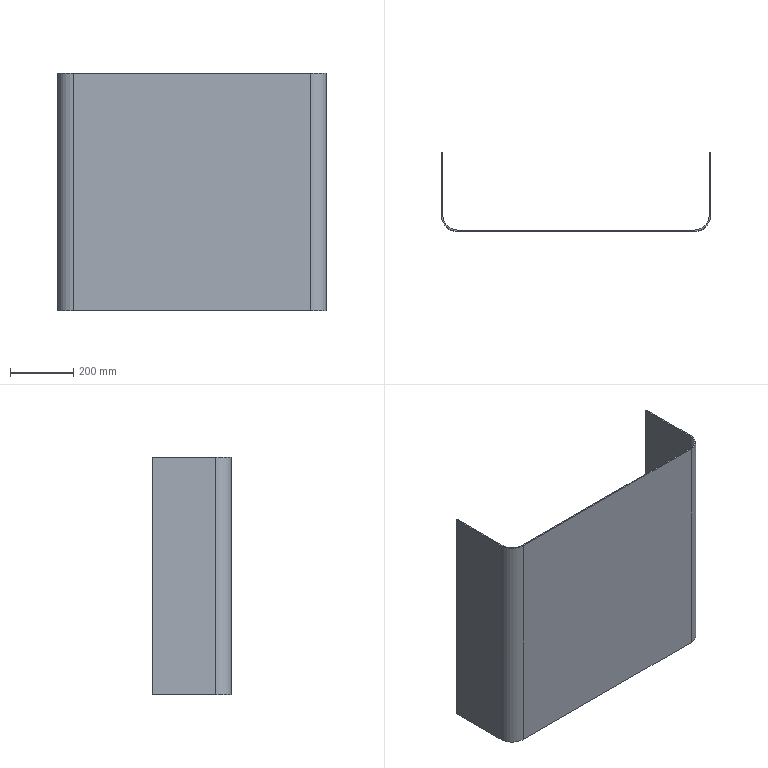Part | SolidWorks | features BaseBody 1 | 1 solid | 14 faces | box 850 x 250 x 750 mm | volume 3902389 mm3 | plane 10 | cylinder 4 | commonest cylinder face diameters 92 x2 100 x2
STEP:
#1=CARTESIAN_POINT('',(375.,0.,0.));
#2=VERTEX_POINT('',#1);
#3=CARTESIAN_POINT('',(375.,0.,750.));
#4=VERTEX_POINT('',#3);
#5=CARTESIAN_POINT('',(375.,0.,375.));
#6=DIRECTION('',(0.,0.,1.));
#7=VECTOR('',#6,1000.);
#8=LINE('',#5,#7);
#9=EDGE_CURVE('',#2,#4,#8,.T.);
#10=ORIENTED_EDGE('',*,*,#9,.T.);
#11=CARTESIAN_POINT('',(-375.,0.,750.));
#12=VERTEX_POINT('',#11);
#13=CARTESIAN_POINT('',(0.,0.,750.));
#14=DIRECTION('',(-1.,0.,0.));
#15=VECTOR('',#14,1000.);
#16=LINE('',#13,#15);
#17=EDGE_CURVE('',#4,#12,#16,.T.);
#18=ORIENTED_EDGE('',*,*,#17,.T.);
#19=CARTESIAN_POINT('',(-375.,0.,0.));
#20=VERTEX_POINT('',#19);
#21=CARTESIAN_POINT('',(-375.,0.,375.));
#22=DIRECTION('',(0.,0.,-1.));
#23=VECTOR('',#22,1000.);
#24=LINE('',#21,#23);
#25=EDGE_CURVE('',#12,#20,#24,.T.);
#26=ORIENTED_EDGE('',*,*,#25,.T.);
#27=CARTESIAN_POINT('',(0.,0.,0.));
#28=DIRECTION('',(1.,0.,0.));
#29=VECTOR('',#28,1000.);
#30=LINE('',#27,#29);
#31=EDGE_CURVE('',#20,#2,#30,.T.);
#32=ORIENTED_EDGE('',*,*,#31,.T.);
#33=EDGE_LOOP('',(#10,#18,#26,#32));
#34=FACE_OUTER_BOUND('',#33,.T.);
#35=CARTESIAN_POINT('',(0.,0.,375.));
#36=DIRECTION('',(0.,-1.,0.));
#37=DIRECTION('',(1.,0.,0.));
#38=AXIS2_PLACEMENT_3D('',#35,#36,#37);
#39=PLANE('',#38);
#40=ADVANCED_FACE('',(#34),#39,.T.);
#41=ORIENTED_EDGE('',*,*,#17,.F.);
#42=CARTESIAN_POINT('',(425.,50.,750.));
#43=VERTEX_POINT('',#42);
#44=CARTESIAN_POINT('',(375.,50.,750.));
#45=DIRECTION('',(0.,0.,-1.));
#46=DIRECTION('',(-1.,0.,0.));
#47=AXIS2_PLACEMENT_3D('',#44,#45,#46);
#48=CIRCLE('',#47,50.);
#49=EDGE_CURVE('',#43,#4,#48,.T.);
#50=ORIENTED_EDGE('',*,*,#49,.F.);
#51=CARTESIAN_POINT('',(425.,250.,750.));
#52=VERTEX_POINT('',#51);
#53=CARTESIAN_POINT('',(425.,-400.021,750.));
#54=DIRECTION('',(0.,-1.,0.));
#55=VECTOR('',#54,1000.);
#56=LINE('',#53,#55);
#57=EDGE_CURVE('',#52,#43,#56,.T.);
#58=ORIENTED_EDGE('',*,*,#57,.F.);
#59=CARTESIAN_POINT('',(421.,250.,750.));
#60=VERTEX_POINT('',#59);
#61=CARTESIAN_POINT('',(421.,250.,750.));
#62=DIRECTION('',(-1.,0.,0.));
#63=VECTOR('',#62,1000.);
#64=LINE('',#61,#63);
#65=EDGE_CURVE('',#52,#60,#64,.T.);
#66=ORIENTED_EDGE('',*,*,#65,.T.);
#67=CARTESIAN_POINT('',(421.,50.,750.));
#68=VERTEX_POINT('',#67);
#69=CARTESIAN_POINT('',(421.,50.,750.));
#70=DIRECTION('',(0.,-1.,0.));
#71=VECTOR('',#70,1000.);
#72=LINE('',#69,#71);
#73=EDGE_CURVE('',#60,#68,#72,.T.);
#74=ORIENTED_EDGE('',*,*,#73,.T.);
#75=CARTESIAN_POINT('',(375.,4.,750.));
#76=VERTEX_POINT('',#75);
#77=CARTESIAN_POINT('',(375.,50.,750.));
#78=DIRECTION('',(0.,0.,-1.));
#79=DIRECTION('',(-1.,0.,0.));
#80=AXIS2_PLACEMENT_3D('',#77,#78,#79);
#81=CIRCLE('',#80,46.);
#82=EDGE_CURVE('',#68,#76,#81,.T.);
#83=ORIENTED_EDGE('',*,*,#82,.T.);
#84=CARTESIAN_POINT('',(-375.,4.,750.));
#85=VERTEX_POINT('',#84);
#86=CARTESIAN_POINT('',(450.021,4.,750.));
#87=DIRECTION('',(-1.,0.,0.));
#88=VECTOR('',#87,1000.);
#89=LINE('',#86,#88);
#90=EDGE_CURVE('',#76,#85,#89,.T.);
#91=ORIENTED_EDGE('',*,*,#90,.T.);
#92=CARTESIAN_POINT('',(-421.,50.,750.));
#93=VERTEX_POINT('',#92);
#94=CARTESIAN_POINT('',(-375.,50.,750.));
#95=DIRECTION('',(0.,0.,-1.));
#96=DIRECTION('',(-1.,0.,0.));
#97=AXIS2_PLACEMENT_3D('',#94,#95,#96);
#98=CIRCLE('',#97,46.);
#99=EDGE_CURVE('',#85,#93,#98,.T.);
#100=ORIENTED_EDGE('',*,*,#99,.T.);
#101=CARTESIAN_POINT('',(-421.,250.,750.));
#102=VERTEX_POINT('',#101);
#103=CARTESIAN_POINT('',(-421.,-850.042,750.));
#104=DIRECTION('',(0.,1.,0.));
#105=VECTOR('',#104,1000.);
#106=LINE('',#103,#105);
#107=EDGE_CURVE('',#93,#102,#106,.T.);
#108=ORIENTED_EDGE('',*,*,#107,.T.);
#109=CARTESIAN_POINT('',(-425.,250.,750.));
#110=VERTEX_POINT('',#109);
#111=CARTESIAN_POINT('',(-421.,250.,750.));
#112=DIRECTION('',(-1.,0.,0.));
#113=VECTOR('',#112,1000.);
#114=LINE('',#111,#113);
#115=EDGE_CURVE('',#102,#110,#114,.T.);
#116=ORIENTED_EDGE('',*,*,#115,.T.);
#117=CARTESIAN_POINT('',(-425.,50.,750.));
#118=VERTEX_POINT('',#117);
#119=CARTESIAN_POINT('',(-425.,-400.021,750.));
#120=DIRECTION('',(0.,1.,0.));
#121=VECTOR('',#120,1000.);
#122=LINE('',#119,#121);
#123=EDGE_CURVE('',#118,#110,#122,.T.);
#124=ORIENTED_EDGE('',*,*,#123,.F.);
#125=CARTESIAN_POINT('',(-375.,50.,750.));
#126=DIRECTION('',(0.,0.,-1.));
#127=DIRECTION('',(-1.,0.,0.));
#128=AXIS2_PLACEMENT_3D('',#125,#126,#127);
#129=CIRCLE('',#128,50.);
#130=EDGE_CURVE('',#12,#118,#129,.T.);
#131=ORIENTED_EDGE('',*,*,#130,.F.);
#132=EDGE_LOOP('',(#41,#50,#58,#66,#74,#83,#91,#100,#108,#116,#124,#131));
#133=FACE_OUTER_BOUND('',#132,.T.);
#134=CARTESIAN_POINT('',(450.021,4.,750.));
#135=DIRECTION('',(0.,0.,1.));
#136=DIRECTION('',(1.,0.,0.));
#137=AXIS2_PLACEMENT_3D('',#134,#135,#136);
#138=PLANE('',#137);
#139=ADVANCED_FACE('',(#133),#138,.T.);
#140=CARTESIAN_POINT('',(425.,50.,0.));
#141=VERTEX_POINT('',#140);
#142=CARTESIAN_POINT('',(425.,50.,375.));
#143=DIRECTION('',(0.,0.,1.));
#144=VECTOR('',#143,1000.);
#145=LINE('',#142,#144);
#146=EDGE_CURVE('',#141,#43,#145,.T.);
#147=ORIENTED_EDGE('',*,*,#146,.T.);
#148=ORIENTED_EDGE('',*,*,#49,.T.);
#149=ORIENTED_EDGE('',*,*,#9,.F.);
#150=CARTESIAN_POINT('',(375.,50.,0.));
#151=DIRECTION('',(0.,0.,1.));
#152=DIRECTION('',(-1.,0.,0.));
#153=AXIS2_PLACEMENT_3D('',#150,#151,#152);
#154=CIRCLE('',#153,50.);
#155=EDGE_CURVE('',#2,#141,#154,.T.);
#156=ORIENTED_EDGE('',*,*,#155,.T.);
#157=EDGE_LOOP('',(#147,#148,#149,#156));
#158=FACE_OUTER_BOUND('',#157,.T.);
#159=CARTESIAN_POINT('',(375.,50.,375.));
#160=DIRECTION('',(0.,0.,-1.));
#161=DIRECTION('',(-1.,0.,0.));
#162=AXIS2_PLACEMENT_3D('',#159,#160,#161);
#163=CYLINDRICAL_SURFACE('',#162,50.);
#164=ADVANCED_FACE('',(#158),#163,.T.);
#165=CARTESIAN_POINT('',(-375.,4.,0.));
#166=VERTEX_POINT('',#165);
#167=CARTESIAN_POINT('',(375.,4.,0.));
#168=VERTEX_POINT('',#167);
#169=CARTESIAN_POINT('',(-450.021,4.,0.));
#170=DIRECTION('',(1.,0.,0.));
#171=VECTOR('',#170,1000.);
#172=LINE('',#169,#171);
#173=EDGE_CURVE('',#166,#168,#172,.T.);
#174=ORIENTED_EDGE('',*,*,#173,.T.);
#175=CARTESIAN_POINT('',(421.,50.,0.));
#176=VERTEX_POINT('',#175);
#177=CARTESIAN_POINT('',(375.,50.,0.));
#178=DIRECTION('',(0.,0.,1.));
#179=DIRECTION('',(-1.,0.,0.));
#180=AXIS2_PLACEMENT_3D('',#177,#178,#179);
#181=CIRCLE('',#180,46.);
#182=EDGE_CURVE('',#168,#176,#181,.T.);
#183=ORIENTED_EDGE('',*,*,#182,.T.);
#184=CARTESIAN_POINT('',(421.,250.,0.));
#185=VERTEX_POINT('',#184);
#186=CARTESIAN_POINT('',(421.,-850.042,0.));
#187=DIRECTION('',(0.,1.,0.));
#188=VECTOR('',#187,1000.);
#189=LINE('',#186,#188);
#190=EDGE_CURVE('',#176,#185,#189,.T.);
#191=ORIENTED_EDGE('',*,*,#190,.T.);
#192=CARTESIAN_POINT('',(425.,250.,0.));
#193=VERTEX_POINT('',#192);
#194=CARTESIAN_POINT('',(421.,250.,0.));
#195=DIRECTION('',(-1.,0.,0.));
#196=VECTOR('',#195,1000.);
#197=LINE('',#194,#196);
#198=EDGE_CURVE('',#193,#185,#197,.T.);
#199=ORIENTED_EDGE('',*,*,#198,.F.);
#200=CARTESIAN_POINT('',(425.,-400.021,0.));
#201=DIRECTION('',(0.,1.,0.));
#202=VECTOR('',#201,1000.);
#203=LINE('',#200,#202);
#204=EDGE_CURVE('',#141,#193,#203,.T.);
#205=ORIENTED_EDGE('',*,*,#204,.F.);
#206=ORIENTED_EDGE('',*,*,#155,.F.);
#207=ORIENTED_EDGE('',*,*,#31,.F.);
#208=CARTESIAN_POINT('',(-425.,50.,0.));
#209=VERTEX_POINT('',#208);
#210=CARTESIAN_POINT('',(-375.,50.,0.));
#211=DIRECTION('',(0.,0.,1.));
#212=DIRECTION('',(-1.,0.,0.));
#213=AXIS2_PLACEMENT_3D('',#210,#211,#212);
#214=CIRCLE('',#213,50.);
#215=EDGE_CURVE('',#209,#20,#214,.T.);
#216=ORIENTED_EDGE('',*,*,#215,.F.);
#217=CARTESIAN_POINT('',(-425.,250.,0.));
#218=VERTEX_POINT('',#217);
#219=CARTESIAN_POINT('',(-425.,-400.021,0.));
#220=DIRECTION('',(0.,-1.,0.));
#221=VECTOR('',#220,1000.);
#222=LINE('',#219,#221);
#223=EDGE_CURVE('',#218,#209,#222,.T.);
#224=ORIENTED_EDGE('',*,*,#223,.F.);
#225=CARTESIAN_POINT('',(-421.,250.,0.));
#226=VERTEX_POINT('',#225);
#227=CARTESIAN_POINT('',(-421.,250.,0.));
#228=DIRECTION('',(1.,0.,0.));
#229=VECTOR('',#228,1000.);
#230=LINE('',#227,#229);
#231=EDGE_CURVE('',#218,#226,#230,.T.);
#232=ORIENTED_EDGE('',*,*,#231,.T.);
#233=CARTESIAN_POINT('',(-421.,50.,0.));
#234=VERTEX_POINT('',#233);
#235=CARTESIAN_POINT('',(-421.,50.,0.));
#236=DIRECTION('',(0.,-1.,0.));
#237=VECTOR('',#236,1000.);
#238=LINE('',#235,#237);
#239=EDGE_CURVE('',#226,#234,#238,.T.);
#240=ORIENTED_EDGE('',*,*,#239,.T.);
#241=CARTESIAN_POINT('',(-375.,50.,0.));
#242=DIRECTION('',(0.,0.,1.));
#243=DIRECTION('',(-1.,0.,0.));
#244=AXIS2_PLACEMENT_3D('',#241,#242,#243);
#245=CIRCLE('',#244,46.);
#246=EDGE_CURVE('',#234,#166,#245,.T.);
#247=ORIENTED_EDGE('',*,*,#246,.T.);
#248=EDGE_LOOP('',(#174,#183,#191,#199,#205,#206,#207,#216,#224,#232,#240,#247));
#249=FACE_OUTER_BOUND('',#248,.T.);
#250=CARTESIAN_POINT('',(-450.021,4.,0.));
#251=DIRECTION('',(0.,0.,-1.));
#252=DIRECTION('',(-1.,0.,0.));
#253=AXIS2_PLACEMENT_3D('',#250,#251,#252);
#254=PLANE('',#253);
#255=ADVANCED_FACE('',(#249),#254,.T.);
#256=ORIENTED_EDGE('',*,*,#25,.F.);
#257=ORIENTED_EDGE('',*,*,#130,.T.);
#258=CARTESIAN_POINT('',(-425.,50.,375.));
#259=DIRECTION('',(0.,0.,-1.));
#260=VECTOR('',#259,1000.);
#261=LINE('',#258,#260);
#262=EDGE_CURVE('',#118,#209,#261,.T.);
#263=ORIENTED_EDGE('',*,*,#262,.T.);
#264=ORIENTED_EDGE('',*,*,#215,.T.);
#265=EDGE_LOOP('',(#256,#257,#263,#264));
#266=FACE_OUTER_BOUND('',#265,.T.);
#267=CARTESIAN_POINT('',(-375.,50.,375.));
#268=DIRECTION('',(0.,0.,-1.));
#269=DIRECTION('',(-1.,0.,0.));
#270=AXIS2_PLACEMENT_3D('',#267,#268,#269);
#271=CYLINDRICAL_SURFACE('',#270,50.);
#272=ADVANCED_FACE('',(#266),#271,.T.);
#273=ORIENTED_EDGE('',*,*,#90,.F.);
#274=CARTESIAN_POINT('',(375.,4.,375.));
#275=DIRECTION('',(0.,0.,1.));
#276=VECTOR('',#275,1000.);
#277=LINE('',#274,#276);
#278=EDGE_CURVE('',#168,#76,#277,.T.);
#279=ORIENTED_EDGE('',*,*,#278,.F.);
#280=ORIENTED_EDGE('',*,*,#173,.F.);
#281=CARTESIAN_POINT('',(-375.,4.,375.));
#282=DIRECTION('',(0.,0.,-1.));
#283=VECTOR('',#282,1000.);
#284=LINE('',#281,#283);
#285=EDGE_CURVE('',#85,#166,#284,.T.);
#286=ORIENTED_EDGE('',*,*,#285,.F.);
#287=EDGE_LOOP('',(#273,#279,#280,#286));
#288=FACE_OUTER_BOUND('',#287,.T.);
#289=CARTESIAN_POINT('',(0.,4.,375.));
#290=DIRECTION('',(0.,-1.,0.));
#291=DIRECTION('',(1.,0.,0.));
#292=AXIS2_PLACEMENT_3D('',#289,#290,#291);
#293=PLANE('',#292);
#294=ADVANCED_FACE('',(#288),#293,.F.);
#295=CARTESIAN_POINT('',(425.,250.,375.));
#296=DIRECTION('',(0.,0.,1.));
#297=VECTOR('',#296,1000.);
#298=LINE('',#295,#297);
#299=EDGE_CURVE('',#193,#52,#298,.T.);
#300=ORIENTED_EDGE('',*,*,#299,.T.);
#301=ORIENTED_EDGE('',*,*,#57,.T.);
#302=ORIENTED_EDGE('',*,*,#146,.F.);
#303=ORIENTED_EDGE('',*,*,#204,.T.);
#304=EDGE_LOOP('',(#300,#301,#302,#303));
#305=FACE_OUTER_BOUND('',#304,.T.);
#306=CARTESIAN_POINT('',(425.,-400.021,375.));
#307=DIRECTION('',(1.,0.,0.));
#308=DIRECTION('',(0.,1.,0.));
#309=AXIS2_PLACEMENT_3D('',#306,#307,#308);
#310=PLANE('',#309);
#311=ADVANCED_FACE('',(#305),#310,.T.);
#312=CARTESIAN_POINT('',(-425.,250.,375.));
#313=DIRECTION('',(0.,0.,-1.));
#314=VECTOR('',#313,1000.);
#315=LINE('',#312,#314);
#316=EDGE_CURVE('',#110,#218,#315,.T.);
#317=ORIENTED_EDGE('',*,*,#316,.T.);
#318=ORIENTED_EDGE('',*,*,#223,.T.);
#319=ORIENTED_EDGE('',*,*,#262,.F.);
#320=ORIENTED_EDGE('',*,*,#123,.T.);
#321=EDGE_LOOP('',(#317,#318,#319,#320));
#322=FACE_OUTER_BOUND('',#321,.T.);
#323=CARTESIAN_POINT('',(-425.,-400.021,375.));
#324=DIRECTION('',(-1.,0.,0.));
#325=DIRECTION('',(0.,-1.,0.));
#326=AXIS2_PLACEMENT_3D('',#323,#324,#325);
#327=PLANE('',#326);
#328=ADVANCED_FACE('',(#322),#327,.T.);
#329=ORIENTED_EDGE('',*,*,#99,.F.);
#330=ORIENTED_EDGE('',*,*,#285,.T.);
#331=ORIENTED_EDGE('',*,*,#246,.F.);
#332=CARTESIAN_POINT('',(-421.,50.,375.));
#333=DIRECTION('',(0.,0.,-1.));
#334=VECTOR('',#333,1000.);
#335=LINE('',#332,#334);
#336=EDGE_CURVE('',#93,#234,#335,.T.);
#337=ORIENTED_EDGE('',*,*,#336,.F.);
#338=EDGE_LOOP('',(#329,#330,#331,#337));
#339=FACE_OUTER_BOUND('',#338,.T.);
#340=CARTESIAN_POINT('',(-375.,50.,375.));
#341=DIRECTION('',(0.,0.,-1.));
#342=DIRECTION('',(-1.,0.,0.));
#343=AXIS2_PLACEMENT_3D('',#340,#341,#342);
#344=CYLINDRICAL_SURFACE('',#343,46.);
#345=ADVANCED_FACE('',(#339),#344,.F.);
#346=ORIENTED_EDGE('',*,*,#82,.F.);
#347=CARTESIAN_POINT('',(421.,50.,375.));
#348=DIRECTION('',(0.,0.,1.));
#349=VECTOR('',#348,1000.);
#350=LINE('',#347,#349);
#351=EDGE_CURVE('',#176,#68,#350,.T.);
#352=ORIENTED_EDGE('',*,*,#351,.F.);
#353=ORIENTED_EDGE('',*,*,#182,.F.);
#354=ORIENTED_EDGE('',*,*,#278,.T.);
#355=EDGE_LOOP('',(#346,#352,#353,#354));
#356=FACE_OUTER_BOUND('',#355,.T.);
#357=CARTESIAN_POINT('',(375.,50.,375.));
#358=DIRECTION('',(0.,0.,-1.));
#359=DIRECTION('',(-1.,0.,0.));
#360=AXIS2_PLACEMENT_3D('',#357,#358,#359);
#361=CYLINDRICAL_SURFACE('',#360,46.);
#362=ADVANCED_FACE('',(#356),#361,.F.);
#363=CARTESIAN_POINT('',(421.,250.,750.));
#364=DIRECTION('',(0.,0.,1.));
#365=VECTOR('',#364,1000.);
#366=LINE('',#363,#365);
#367=EDGE_CURVE('',#185,#60,#366,.T.);
#368=ORIENTED_EDGE('',*,*,#367,.T.);
#369=ORIENTED_EDGE('',*,*,#65,.F.);
#370=ORIENTED_EDGE('',*,*,#299,.F.);
#371=ORIENTED_EDGE('',*,*,#198,.T.);
#372=EDGE_LOOP('',(#368,#369,#370,#371));
#373=FACE_OUTER_BOUND('',#372,.T.);
#374=CARTESIAN_POINT('',(421.,250.,750.));
#375=DIRECTION('',(0.,1.,0.));
#376=DIRECTION('',(0.,0.,1.));
#377=AXIS2_PLACEMENT_3D('',#374,#375,#376);
#378=PLANE('',#377);
#379=ADVANCED_FACE('',(#373),#378,.T.);
#380=CARTESIAN_POINT('',(-421.,250.,0.));
#381=DIRECTION('',(0.,0.,-1.));
#382=VECTOR('',#381,1000.);
#383=LINE('',#380,#382);
#384=EDGE_CURVE('',#102,#226,#383,.T.);
#385=ORIENTED_EDGE('',*,*,#384,.T.);
#386=ORIENTED_EDGE('',*,*,#231,.F.);
#387=ORIENTED_EDGE('',*,*,#316,.F.);
#388=ORIENTED_EDGE('',*,*,#115,.F.);
#389=EDGE_LOOP('',(#385,#386,#387,#388));
#390=FACE_OUTER_BOUND('',#389,.T.);
#391=CARTESIAN_POINT('',(-421.,250.,0.));
#392=DIRECTION('',(0.,1.,0.));
#393=DIRECTION('',(-1.,0.,0.));
#394=AXIS2_PLACEMENT_3D('',#391,#392,#393);
#395=PLANE('',#394);
#396=ADVANCED_FACE('',(#390),#395,.T.);
#397=ORIENTED_EDGE('',*,*,#239,.F.);
#398=ORIENTED_EDGE('',*,*,#384,.F.);
#399=ORIENTED_EDGE('',*,*,#107,.F.);
#400=ORIENTED_EDGE('',*,*,#336,.T.);
#401=EDGE_LOOP('',(#397,#398,#399,#400));
#402=FACE_OUTER_BOUND('',#401,.T.);
#403=CARTESIAN_POINT('',(-421.,-400.021,375.));
#404=DIRECTION('',(-1.,0.,0.));
#405=DIRECTION('',(0.,-1.,0.));
#406=AXIS2_PLACEMENT_3D('',#403,#404,#405);
#407=PLANE('',#406);
#408=ADVANCED_FACE('',(#402),#407,.F.);
#409=ORIENTED_EDGE('',*,*,#73,.F.);
#410=ORIENTED_EDGE('',*,*,#367,.F.);
#411=ORIENTED_EDGE('',*,*,#190,.F.);
#412=ORIENTED_EDGE('',*,*,#351,.T.);
#413=EDGE_LOOP('',(#409,#410,#411,#412));
#414=FACE_OUTER_BOUND('',#413,.T.);
#415=CARTESIAN_POINT('',(421.,-400.021,375.));
#416=DIRECTION('',(1.,0.,0.));
#417=DIRECTION('',(0.,1.,0.));
#418=AXIS2_PLACEMENT_3D('',#415,#416,#417);
#419=PLANE('',#418);
#420=ADVANCED_FACE('',(#414),#419,.F.);
#421=CLOSED_SHELL('',(#40,#139,#164,#255,#272,#294,#311,#328,#345,#362,#379,#396,#408,#420));
#422=MANIFOLD_SOLID_BREP('',#421);
#423=CARTESIAN_POINT('',(0.,0.,0.));
#424=DIRECTION('',(0.,0.,1.));
#425=DIRECTION('',(1.,0.,0.));
#426=AXIS2_PLACEMENT_3D('',#423,#424,#425);
#427=(LENGTH_UNIT()NAMED_UNIT(*)SI_UNIT(.MILLI.,.METRE.));
#428=UNCERTAINTY_MEASURE_WITH_UNIT(LENGTH_MEASURE(0.00001),#427,'','');
#429=(NAMED_UNIT(*)PLANE_ANGLE_UNIT()SI_UNIT($,.RADIAN.));
#430=(NAMED_UNIT(*)SI_UNIT($,.STERADIAN.)SOLID_ANGLE_UNIT());
#431=(GEOMETRIC_REPRESENTATION_CONTEXT(3)GLOBAL_UNCERTAINTY_ASSIGNED_CONTEXT((#428))GLOBAL_UNIT_ASSIGNED_CONTEXT((#427,#429,#430))REPRESENTATION_CONTEXT('',''));
#432=ADVANCED_BREP_SHAPE_REPRESENTATION('',(#422,#426),#431);